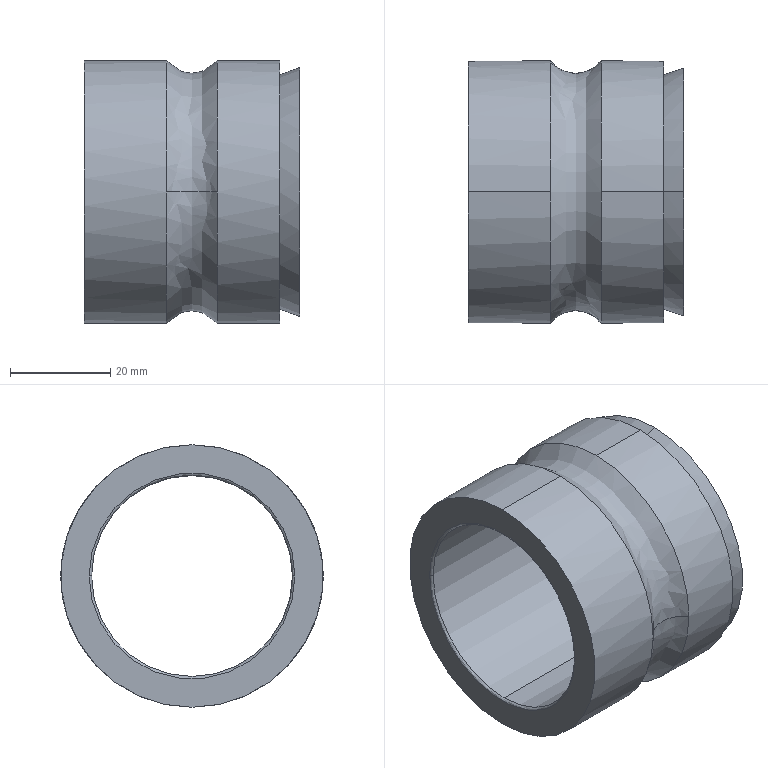Part | SolidWorks | features BaseBody 1 | 1 solid | 17 faces | box 42.9 x 52.3 x 52.3 mm | volume 34134 mm3 | spline 10 | cylinder 4 | plane 3 | commonest cylinder face diameters 52.3 x4
STEP:
#1=CARTESIAN_POINT('',(5.05,48.85,49.2));
#2=VERTEX_POINT('',#1);
#3=CARTESIAN_POINT('',(5.05,75.,23.05));
#4=VERTEX_POINT('',#3);
#5=CARTESIAN_POINT('',(5.05,75.,49.2));
#6=DIRECTION('',(1.,0.,0.));
#7=DIRECTION('',(0.,0.,1.));
#8=AXIS2_PLACEMENT_3D('',#5,#6,#7);
#9=CIRCLE('',#8,26.15);
#10=EDGE_CURVE('',#2,#4,#9,.T.);
#11=ORIENTED_EDGE('',*,*,#10,.F.);
#12=CARTESIAN_POINT('',(-5.05,48.85,49.2));
#13=VERTEX_POINT('',#12);
#14=CARTESIAN_POINT('',(0.,45.,49.2));
#15=DIRECTION('',(0.,0.,1.));
#16=DIRECTION('',(0.,-1.,0.));
#17=AXIS2_PLACEMENT_3D('',#14,#15,#16);
#18=CIRCLE('',#17,6.35);
#19=EDGE_CURVE('',#2,#13,#18,.T.);
#20=ORIENTED_EDGE('',*,*,#19,.T.);
#21=CARTESIAN_POINT('',(-5.05,75.,23.05));
#22=VERTEX_POINT('',#21);
#23=CARTESIAN_POINT('',(-5.05,75.,49.2));
#24=DIRECTION('',(1.,0.,0.));
#25=DIRECTION('',(0.,0.,1.));
#26=AXIS2_PLACEMENT_3D('',#23,#24,#25);
#27=CIRCLE('',#26,26.15);
#28=EDGE_CURVE('',#13,#22,#27,.T.);
#29=ORIENTED_EDGE('',*,*,#28,.T.);
#30=CARTESIAN_POINT('',(-5.05,101.15,49.2));
#31=VERTEX_POINT('',#30);
#32=CARTESIAN_POINT('',(-5.05,75.,49.2));
#33=DIRECTION('',(1.,0.,0.));
#34=DIRECTION('',(0.,0.,1.));
#35=AXIS2_PLACEMENT_3D('',#32,#33,#34);
#36=CIRCLE('',#35,26.15);
#37=EDGE_CURVE('',#22,#31,#36,.T.);
#38=ORIENTED_EDGE('',*,*,#37,.T.);
#39=CARTESIAN_POINT('',(5.05,101.15,49.2));
#40=VERTEX_POINT('',#39);
#41=CARTESIAN_POINT('',(0.,105.,49.2));
#42=DIRECTION('',(0.,0.,-1.));
#43=DIRECTION('',(0.,1.,0.));
#44=AXIS2_PLACEMENT_3D('',#41,#42,#43);
#45=CIRCLE('',#44,6.35);
#46=EDGE_CURVE('',#40,#31,#45,.T.);
#47=ORIENTED_EDGE('',*,*,#46,.F.);
#48=CARTESIAN_POINT('',(5.05,75.,49.2));
#49=DIRECTION('',(1.,0.,0.));
#50=DIRECTION('',(0.,0.,1.));
#51=AXIS2_PLACEMENT_3D('',#48,#49,#50);
#52=CIRCLE('',#51,26.15);
#53=EDGE_CURVE('',#4,#40,#52,.T.);
#54=ORIENTED_EDGE('',*,*,#53,.F.);
#55=EDGE_LOOP('',(#11,#20,#29,#38,#47,#54));
#56=FACE_OUTER_BOUND('',#55,.T.);
#57=CARTESIAN_POINT('',(5.05,48.85,49.2));
#58=CARTESIAN_POINT('',(5.05,48.85,-3.1));
#59=CARTESIAN_POINT('',(5.05,101.15,-3.1));
#60=CARTESIAN_POINT('',(5.05,101.15,49.2));
#61=CARTESIAN_POINT('',(2.282,52.48,49.2));
#62=CARTESIAN_POINT('',(2.282,52.48,4.16));
#63=CARTESIAN_POINT('',(2.282,97.52,4.16));
#64=CARTESIAN_POINT('',(2.282,97.52,49.2));
#65=CARTESIAN_POINT('',(-2.282,52.48,49.2));
#66=CARTESIAN_POINT('',(-2.282,52.48,4.16));
#67=CARTESIAN_POINT('',(-2.282,97.52,4.16));
#68=CARTESIAN_POINT('',(-2.282,97.52,49.2));
#69=CARTESIAN_POINT('',(-5.05,48.85,49.2));
#70=CARTESIAN_POINT('',(-5.05,48.85,-3.1));
#71=CARTESIAN_POINT('',(-5.05,101.15,-3.1));
#72=CARTESIAN_POINT('',(-5.05,101.15,49.2));
#73=(BOUNDED_SURFACE()B_SPLINE_SURFACE(3,3,((#57,#58,#59,#60),(#61,#62,#63,#64),(#65,#66,#67,#68),(#69,#70,#71,#72)),.UNSPECIFIED.,.F.,.F.,.F.)B_SPLINE_SURFACE_WITH_KNOTS((4,4),(4,4),(0.,1.),(0.,1.),.UNSPECIFIED.)GEOMETRIC_REPRESENTATION_ITEM()RATIONAL_B_SPLINE_SURFACE(((1.,0.3333,0.3333,1.),(0.7375,0.2458,0.2458,0.7375),(0.7375,0.2458,0.2458,0.7375),(1.,0.3333,0.3333,1.)))REPRESENTATION_ITEM('')SURFACE());
#74=ADVANCED_FACE('',(#56),#73,.T.);
#75=CARTESIAN_POINT('',(21.5,75.,24.419));
#76=VERTEX_POINT('',#75);
#77=CARTESIAN_POINT('',(21.5,75.,73.981));
#78=VERTEX_POINT('',#77);
#79=CARTESIAN_POINT('',(21.5,75.,49.2));
#80=DIRECTION('',(1.,0.,0.));
#81=DIRECTION('',(0.,0.,1.));
#82=AXIS2_PLACEMENT_3D('',#79,#80,#81);
#83=CIRCLE('',#82,24.781);
#84=EDGE_CURVE('',#76,#78,#83,.T.);
#85=ORIENTED_EDGE('',*,*,#84,.F.);
#86=CARTESIAN_POINT('',(17.5,75.,25.875));
#87=VERTEX_POINT('',#86);
#88=CARTESIAN_POINT('',(19.5,75.,25.147));
#89=DIRECTION('',(-0.9397,0.,0.342));
#90=VECTOR('',#89,1000.);
#91=LINE('',#88,#90);
#92=EDGE_CURVE('',#76,#87,#91,.T.);
#93=ORIENTED_EDGE('',*,*,#92,.T.);
#94=CARTESIAN_POINT('',(17.5,75.,72.525));
#95=VERTEX_POINT('',#94);
#96=CARTESIAN_POINT('',(17.5,75.,49.2));
#97=DIRECTION('',(1.,0.,0.));
#98=DIRECTION('',(0.,0.,1.));
#99=AXIS2_PLACEMENT_3D('',#96,#97,#98);
#100=CIRCLE('',#99,23.325);
#101=EDGE_CURVE('',#87,#95,#100,.T.);
#102=ORIENTED_EDGE('',*,*,#101,.T.);
#103=CARTESIAN_POINT('',(19.5,75.,73.253));
#104=DIRECTION('',(-0.9397,0.,-0.342));
#105=VECTOR('',#104,1000.);
#106=LINE('',#103,#105);
#107=EDGE_CURVE('',#78,#95,#106,.T.);
#108=ORIENTED_EDGE('',*,*,#107,.F.);
#109=EDGE_LOOP('',(#85,#93,#102,#108));
#110=FACE_OUTER_BOUND('',#109,.T.);
#111=CARTESIAN_POINT('',(21.5,75.,24.419));
#112=CARTESIAN_POINT('',(21.5,124.562,24.419));
#113=CARTESIAN_POINT('',(21.5,124.562,73.981));
#114=CARTESIAN_POINT('',(21.5,75.,73.981));
#115=CARTESIAN_POINT('',(17.5,75.,25.875));
#116=CARTESIAN_POINT('',(17.5,121.65,25.875));
#117=CARTESIAN_POINT('',(17.5,121.65,72.525));
#118=CARTESIAN_POINT('',(17.5,75.,72.525));
#119=(BOUNDED_SURFACE()B_SPLINE_SURFACE(1,3,((#111,#112,#113,#114),(#115,#116,#117,#118)),.UNSPECIFIED.,.F.,.F.,.F.)B_SPLINE_SURFACE_WITH_KNOTS((2,2),(4,4),(0.,1.),(0.,1.),.UNSPECIFIED.)GEOMETRIC_REPRESENTATION_ITEM()RATIONAL_B_SPLINE_SURFACE(((1.,0.3333,0.3333,1.),(1.,0.3333,0.3333,1.)))REPRESENTATION_ITEM('')SURFACE());
#120=ADVANCED_FACE('',(#110),#119,.T.);
#121=CARTESIAN_POINT('',(21.,55.,49.2));
#122=VERTEX_POINT('',#121);
#123=CARTESIAN_POINT('',(21.,75.,29.2));
#124=VERTEX_POINT('',#123);
#125=CARTESIAN_POINT('',(21.,75.,49.2));
#126=DIRECTION('',(1.,0.,0.));
#127=DIRECTION('',(0.,0.,1.));
#128=AXIS2_PLACEMENT_3D('',#125,#126,#127);
#129=CIRCLE('',#128,20.);
#130=EDGE_CURVE('',#122,#124,#129,.T.);
#131=ORIENTED_EDGE('',*,*,#130,.F.);
#132=CARTESIAN_POINT('',(21.5,54.5,49.2));
#133=VERTEX_POINT('',#132);
#134=CARTESIAN_POINT('',(21.,54.5,49.2));
#135=DIRECTION('',(0.,0.,-1.));
#136=DIRECTION('',(0.,-1.,0.));
#137=AXIS2_PLACEMENT_3D('',#134,#135,#136);
#138=CIRCLE('',#137,0.5);
#139=EDGE_CURVE('',#122,#133,#138,.T.);
#140=ORIENTED_EDGE('',*,*,#139,.T.);
#141=CARTESIAN_POINT('',(21.5,95.5,49.2));
#142=VERTEX_POINT('',#141);
#143=CARTESIAN_POINT('',(21.5,75.,49.2));
#144=DIRECTION('',(1.,0.,0.));
#145=DIRECTION('',(0.,0.,1.));
#146=AXIS2_PLACEMENT_3D('',#143,#144,#145);
#147=CIRCLE('',#146,20.5);
#148=EDGE_CURVE('',#133,#142,#147,.T.);
#149=ORIENTED_EDGE('',*,*,#148,.T.);
#150=CARTESIAN_POINT('',(21.,95.,49.2));
#151=VERTEX_POINT('',#150);
#152=CARTESIAN_POINT('',(21.,95.5,49.2));
#153=DIRECTION('',(0.,0.,1.));
#154=DIRECTION('',(0.,1.,0.));
#155=AXIS2_PLACEMENT_3D('',#152,#153,#154);
#156=CIRCLE('',#155,0.5);
#157=EDGE_CURVE('',#151,#142,#156,.T.);
#158=ORIENTED_EDGE('',*,*,#157,.F.);
#159=CARTESIAN_POINT('',(21.,75.,49.2));
#160=DIRECTION('',(1.,0.,0.));
#161=DIRECTION('',(0.,0.,1.));
#162=AXIS2_PLACEMENT_3D('',#159,#160,#161);
#163=CIRCLE('',#162,20.);
#164=EDGE_CURVE('',#124,#151,#163,.T.);
#165=ORIENTED_EDGE('',*,*,#164,.F.);
#166=EDGE_LOOP('',(#131,#140,#149,#158,#165));
#167=FACE_OUTER_BOUND('',#166,.T.);
#168=CARTESIAN_POINT('',(21.,55.,49.2));
#169=CARTESIAN_POINT('',(21.,55.,9.2));
#170=CARTESIAN_POINT('',(21.,95.,9.2));
#171=CARTESIAN_POINT('',(21.,95.,49.2));
#172=CARTESIAN_POINT('',(21.293,55.,49.2));
#173=CARTESIAN_POINT('',(21.293,55.,9.2));
#174=CARTESIAN_POINT('',(21.293,95.,9.2));
#175=CARTESIAN_POINT('',(21.293,95.,49.2));
#176=CARTESIAN_POINT('',(21.5,54.793,49.2));
#177=CARTESIAN_POINT('',(21.5,54.793,8.786));
#178=CARTESIAN_POINT('',(21.5,95.207,8.786));
#179=CARTESIAN_POINT('',(21.5,95.207,49.2));
#180=CARTESIAN_POINT('',(21.5,54.5,49.2));
#181=CARTESIAN_POINT('',(21.5,54.5,8.2));
#182=CARTESIAN_POINT('',(21.5,95.5,8.2));
#183=CARTESIAN_POINT('',(21.5,95.5,49.2));
#184=(BOUNDED_SURFACE()B_SPLINE_SURFACE(3,3,((#168,#169,#170,#171),(#172,#173,#174,#175),(#176,#177,#178,#179),(#180,#181,#182,#183)),.UNSPECIFIED.,.F.,.F.,.F.)B_SPLINE_SURFACE_WITH_KNOTS((4,4),(4,4),(0.,1.),(0.,1.),.UNSPECIFIED.)GEOMETRIC_REPRESENTATION_ITEM()RATIONAL_B_SPLINE_SURFACE(((1.,0.3333,0.3333,1.),(0.8047,0.2682,0.2682,0.8047),(0.8047,0.2682,0.2682,0.8047),(1.,0.3333,0.3333,1.)))REPRESENTATION_ITEM('')SURFACE());
#185=ADVANCED_FACE('',(#167),#184,.T.);
#186=CARTESIAN_POINT('',(-21.4,54.5,49.2));
#187=VERTEX_POINT('',#186);
#188=CARTESIAN_POINT('',(-21.4,95.5,49.2));
#189=VERTEX_POINT('',#188);
#190=CARTESIAN_POINT('',(-21.4,75.,49.2));
#191=DIRECTION('',(1.,0.,0.));
#192=DIRECTION('',(0.,0.,1.));
#193=AXIS2_PLACEMENT_3D('',#190,#191,#192);
#194=CIRCLE('',#193,20.5);
#195=EDGE_CURVE('',#187,#189,#194,.T.);
#196=ORIENTED_EDGE('',*,*,#195,.F.);
#197=CARTESIAN_POINT('',(-20.9,55.,49.2));
#198=VERTEX_POINT('',#197);
#199=CARTESIAN_POINT('',(-20.9,54.5,49.2));
#200=DIRECTION('',(0.,0.,-1.));
#201=DIRECTION('',(0.,-1.,0.));
#202=AXIS2_PLACEMENT_3D('',#199,#200,#201);
#203=CIRCLE('',#202,0.5);
#204=EDGE_CURVE('',#187,#198,#203,.T.);
#205=ORIENTED_EDGE('',*,*,#204,.T.);
#206=CARTESIAN_POINT('',(-20.9,75.,29.2));
#207=VERTEX_POINT('',#206);
#208=CARTESIAN_POINT('',(-20.9,75.,49.2));
#209=DIRECTION('',(1.,0.,0.));
#210=DIRECTION('',(0.,0.,1.));
#211=AXIS2_PLACEMENT_3D('',#208,#209,#210);
#212=CIRCLE('',#211,20.);
#213=EDGE_CURVE('',#198,#207,#212,.T.);
#214=ORIENTED_EDGE('',*,*,#213,.T.);
#215=CARTESIAN_POINT('',(-20.9,95.,49.2));
#216=VERTEX_POINT('',#215);
#217=CARTESIAN_POINT('',(-20.9,75.,49.2));
#218=DIRECTION('',(1.,0.,0.));
#219=DIRECTION('',(0.,0.,1.));
#220=AXIS2_PLACEMENT_3D('',#217,#218,#219);
#221=CIRCLE('',#220,20.);
#222=EDGE_CURVE('',#207,#216,#221,.T.);
#223=ORIENTED_EDGE('',*,*,#222,.T.);
#224=CARTESIAN_POINT('',(-20.9,95.5,49.2));
#225=DIRECTION('',(0.,0.,1.));
#226=DIRECTION('',(0.,1.,0.));
#227=AXIS2_PLACEMENT_3D('',#224,#225,#226);
#228=CIRCLE('',#227,0.5);
#229=EDGE_CURVE('',#189,#216,#228,.T.);
#230=ORIENTED_EDGE('',*,*,#229,.F.);
#231=EDGE_LOOP('',(#196,#205,#214,#223,#230));
#232=FACE_OUTER_BOUND('',#231,.T.);
#233=CARTESIAN_POINT('',(-21.4,54.5,49.2));
#234=CARTESIAN_POINT('',(-21.4,54.5,8.2));
#235=CARTESIAN_POINT('',(-21.4,95.5,8.2));
#236=CARTESIAN_POINT('',(-21.4,95.5,49.2));
#237=CARTESIAN_POINT('',(-21.4,54.793,49.2));
#238=CARTESIAN_POINT('',(-21.4,54.793,8.786));
#239=CARTESIAN_POINT('',(-21.4,95.207,8.786));
#240=CARTESIAN_POINT('',(-21.4,95.207,49.2));
#241=CARTESIAN_POINT('',(-21.193,55.,49.2));
#242=CARTESIAN_POINT('',(-21.193,55.,9.2));
#243=CARTESIAN_POINT('',(-21.193,95.,9.2));
#244=CARTESIAN_POINT('',(-21.193,95.,49.2));
#245=CARTESIAN_POINT('',(-20.9,55.,49.2));
#246=CARTESIAN_POINT('',(-20.9,55.,9.2));
#247=CARTESIAN_POINT('',(-20.9,95.,9.2));
#248=CARTESIAN_POINT('',(-20.9,95.,49.2));
#249=(BOUNDED_SURFACE()B_SPLINE_SURFACE(3,3,((#233,#234,#235,#236),(#237,#238,#239,#240),(#241,#242,#243,#244),(#245,#246,#247,#248)),.UNSPECIFIED.,.F.,.F.,.T.)B_SPLINE_SURFACE_WITH_KNOTS((4,4),(4,4),(0.,1.),(0.,1.),.UNSPECIFIED.)GEOMETRIC_REPRESENTATION_ITEM()RATIONAL_B_SPLINE_SURFACE(((1.,0.3333,0.3333,1.),(0.8047,0.2682,0.2682,0.8047),(0.8047,0.2682,0.2682,0.8047),(1.,0.3333,0.3333,1.)))REPRESENTATION_ITEM('')SURFACE());
#250=ADVANCED_FACE('',(#232),#249,.T.);
#251=CARTESIAN_POINT('',(-21.4,75.,23.05));
#252=VERTEX_POINT('',#251);
#253=CARTESIAN_POINT('',(-21.4,75.,75.35));
#254=VERTEX_POINT('',#253);
#255=CARTESIAN_POINT('',(-21.4,75.,49.2));
#256=DIRECTION('',(1.,0.,0.));
#257=DIRECTION('',(0.,0.,1.));
#258=AXIS2_PLACEMENT_3D('',#255,#256,#257);
#259=CIRCLE('',#258,26.15);
#260=EDGE_CURVE('',#252,#254,#259,.T.);
#261=ORIENTED_EDGE('',*,*,#260,.T.);
#262=CARTESIAN_POINT('',(-5.05,75.,75.35));
#263=VERTEX_POINT('',#262);
#264=CARTESIAN_POINT('',(-13.225,75.,75.35));
#265=DIRECTION('',(1.,0.,0.));
#266=VECTOR('',#265,1000.);
#267=LINE('',#264,#266);
#268=EDGE_CURVE('',#254,#263,#267,.T.);
#269=ORIENTED_EDGE('',*,*,#268,.T.);
#270=CARTESIAN_POINT('',(-5.05,75.,49.2));
#271=DIRECTION('',(1.,0.,0.));
#272=DIRECTION('',(0.,0.,1.));
#273=AXIS2_PLACEMENT_3D('',#270,#271,#272);
#274=CIRCLE('',#273,26.15);
#275=EDGE_CURVE('',#31,#263,#274,.T.);
#276=ORIENTED_EDGE('',*,*,#275,.F.);
#277=ORIENTED_EDGE('',*,*,#37,.F.);
#278=CARTESIAN_POINT('',(-13.225,75.,23.05));
#279=DIRECTION('',(1.,0.,0.));
#280=VECTOR('',#279,1000.);
#281=LINE('',#278,#280);
#282=EDGE_CURVE('',#252,#22,#281,.T.);
#283=ORIENTED_EDGE('',*,*,#282,.F.);
#284=EDGE_LOOP('',(#261,#269,#276,#277,#283));
#285=FACE_OUTER_BOUND('',#284,.T.);
#286=CARTESIAN_POINT('',(-13.225,75.,49.2));
#287=DIRECTION('',(1.,0.,0.));
#288=DIRECTION('',(0.,0.,-1.));
#289=AXIS2_PLACEMENT_3D('',#286,#287,#288);
#290=CYLINDRICAL_SURFACE('',#289,26.15);
#291=ADVANCED_FACE('',(#285),#290,.T.);
#292=ORIENTED_EDGE('',*,*,#53,.T.);
#293=CARTESIAN_POINT('',(5.05,75.,75.35));
#294=VERTEX_POINT('',#293);
#295=CARTESIAN_POINT('',(5.05,75.,49.2));
#296=DIRECTION('',(1.,0.,0.));
#297=DIRECTION('',(0.,0.,1.));
#298=AXIS2_PLACEMENT_3D('',#295,#296,#297);
#299=CIRCLE('',#298,26.15);
#300=EDGE_CURVE('',#40,#294,#299,.T.);
#301=ORIENTED_EDGE('',*,*,#300,.T.);
#302=CARTESIAN_POINT('',(17.5,75.,75.35));
#303=VERTEX_POINT('',#302);
#304=CARTESIAN_POINT('',(11.275,75.,75.35));
#305=DIRECTION('',(1.,0.,0.));
#306=VECTOR('',#305,1000.);
#307=LINE('',#304,#306);
#308=EDGE_CURVE('',#294,#303,#307,.T.);
#309=ORIENTED_EDGE('',*,*,#308,.T.);
#310=CARTESIAN_POINT('',(17.5,75.,23.05));
#311=VERTEX_POINT('',#310);
#312=CARTESIAN_POINT('',(17.5,75.,49.2));
#313=DIRECTION('',(1.,0.,0.));
#314=DIRECTION('',(0.,0.,1.));
#315=AXIS2_PLACEMENT_3D('',#312,#313,#314);
#316=CIRCLE('',#315,26.15);
#317=EDGE_CURVE('',#311,#303,#316,.T.);
#318=ORIENTED_EDGE('',*,*,#317,.F.);
#319=CARTESIAN_POINT('',(11.275,75.,23.05));
#320=DIRECTION('',(1.,0.,0.));
#321=VECTOR('',#320,1000.);
#322=LINE('',#319,#321);
#323=EDGE_CURVE('',#4,#311,#322,.T.);
#324=ORIENTED_EDGE('',*,*,#323,.F.);
#325=EDGE_LOOP('',(#292,#301,#309,#318,#324));
#326=FACE_OUTER_BOUND('',#325,.T.);
#327=CARTESIAN_POINT('',(11.275,75.,49.2));
#328=DIRECTION('',(1.,0.,0.));
#329=DIRECTION('',(0.,0.,-1.));
#330=AXIS2_PLACEMENT_3D('',#327,#328,#329);
#331=CYLINDRICAL_SURFACE('',#330,26.15);
#332=ADVANCED_FACE('',(#326),#331,.T.);
#333=ORIENTED_EDGE('',*,*,#222,.F.);
#334=CARTESIAN_POINT('',(0.05,75.,29.2));
#335=DIRECTION('',(1.,0.,0.));
#336=VECTOR('',#335,1000.);
#337=LINE('',#334,#336);
#338=EDGE_CURVE('',#207,#124,#337,.T.);
#339=ORIENTED_EDGE('',*,*,#338,.T.);
#340=ORIENTED_EDGE('',*,*,#164,.T.);
#341=CARTESIAN_POINT('',(21.,75.,69.2));
#342=VERTEX_POINT('',#341);
#343=CARTESIAN_POINT('',(21.,75.,49.2));
#344=DIRECTION('',(1.,0.,0.));
#345=DIRECTION('',(0.,0.,1.));
#346=AXIS2_PLACEMENT_3D('',#343,#344,#345);
#347=CIRCLE('',#346,20.);
#348=EDGE_CURVE('',#151,#342,#347,.T.);
#349=ORIENTED_EDGE('',*,*,#348,.T.);
#350=CARTESIAN_POINT('',(-20.9,75.,69.2));
#351=VERTEX_POINT('',#350);
#352=CARTESIAN_POINT('',(0.05,75.,69.2));
#353=DIRECTION('',(1.,0.,0.));
#354=VECTOR('',#353,1000.);
#355=LINE('',#352,#354);
#356=EDGE_CURVE('',#351,#342,#355,.T.);
#357=ORIENTED_EDGE('',*,*,#356,.F.);
#358=CARTESIAN_POINT('',(-20.9,75.,49.2));
#359=DIRECTION('',(1.,0.,0.));
#360=DIRECTION('',(0.,0.,1.));
#361=AXIS2_PLACEMENT_3D('',#358,#359,#360);
#362=CIRCLE('',#361,20.);
#363=EDGE_CURVE('',#216,#351,#362,.T.);
#364=ORIENTED_EDGE('',*,*,#363,.F.);
#365=EDGE_LOOP('',(#333,#339,#340,#349,#357,#364));
#366=FACE_OUTER_BOUND('',#365,.T.);
#367=CARTESIAN_POINT('',(-20.9,75.,69.2));
#368=CARTESIAN_POINT('',(21.,75.,69.2));
#369=CARTESIAN_POINT('',(-20.9,115.,69.2));
#370=CARTESIAN_POINT('',(21.,115.,69.2));
#371=CARTESIAN_POINT('',(-20.9,115.,29.2));
#372=CARTESIAN_POINT('',(21.,115.,29.2));
#373=CARTESIAN_POINT('',(-20.9,75.,29.2));
#374=CARTESIAN_POINT('',(21.,75.,29.2));
#375=(BOUNDED_SURFACE()B_SPLINE_SURFACE(3,1,((#367,#368),(#369,#370),(#371,#372),(#373,#374)),.UNSPECIFIED.,.F.,.F.,.F.)B_SPLINE_SURFACE_WITH_KNOTS((4,4),(2,2),(0.,1.),(0.,1.),.UNSPECIFIED.)GEOMETRIC_REPRESENTATION_ITEM()RATIONAL_B_SPLINE_SURFACE(((1.,1.),(0.3333,0.3333),(0.3333,0.3333),(1.,1.)))REPRESENTATION_ITEM('')SURFACE());
#376=ADVANCED_FACE('',(#366),#375,.T.);
#377=CARTESIAN_POINT('',(-21.4,75.,49.2));
#378=DIRECTION('',(1.,0.,0.));
#379=DIRECTION('',(0.,0.,1.));
#380=AXIS2_PLACEMENT_3D('',#377,#378,#379);
#381=CIRCLE('',#380,20.5);
#382=EDGE_CURVE('',#189,#187,#381,.T.);
#383=ORIENTED_EDGE('',*,*,#382,.T.);
#384=ORIENTED_EDGE('',*,*,#195,.T.);
#385=EDGE_LOOP('',(#383,#384));
#386=FACE_BOUND('',#385,.T.);
#387=ORIENTED_EDGE('',*,*,#260,.F.);
#388=CARTESIAN_POINT('',(-21.4,75.,49.2));
#389=DIRECTION('',(1.,0.,0.));
#390=DIRECTION('',(0.,0.,1.));
#391=AXIS2_PLACEMENT_3D('',#388,#389,#390);
#392=CIRCLE('',#391,26.15);
#393=EDGE_CURVE('',#254,#252,#392,.T.);
#394=ORIENTED_EDGE('',*,*,#393,.F.);
#395=EDGE_LOOP('',(#387,#394));
#396=FACE_OUTER_BOUND('',#395,.T.);
#397=CARTESIAN_POINT('',(-21.4,75.,72.525));
#398=DIRECTION('',(-1.,0.,0.));
#399=DIRECTION('',(0.,0.,1.));
#400=AXIS2_PLACEMENT_3D('',#397,#398,#399);
#401=PLANE('',#400);
#402=ADVANCED_FACE('',(#386,#396),#401,.T.);
#403=ORIENTED_EDGE('',*,*,#204,.F.);
#404=ORIENTED_EDGE('',*,*,#382,.F.);
#405=ORIENTED_EDGE('',*,*,#229,.T.);
#406=ORIENTED_EDGE('',*,*,#363,.T.);
#407=CARTESIAN_POINT('',(-20.9,75.,49.2));
#408=DIRECTION('',(1.,0.,0.));
#409=DIRECTION('',(0.,0.,1.));
#410=AXIS2_PLACEMENT_3D('',#407,#408,#409);
#411=CIRCLE('',#410,20.);
#412=EDGE_CURVE('',#351,#198,#411,.T.);
#413=ORIENTED_EDGE('',*,*,#412,.T.);
#414=EDGE_LOOP('',(#403,#404,#405,#406,#413));
#415=FACE_OUTER_BOUND('',#414,.T.);
#416=CARTESIAN_POINT('',(-21.4,95.5,49.2));
#417=CARTESIAN_POINT('',(-21.4,95.5,90.2));
#418=CARTESIAN_POINT('',(-21.4,54.5,90.2));
#419=CARTESIAN_POINT('',(-21.4,54.5,49.2));
#420=CARTESIAN_POINT('',(-21.4,95.207,49.2));
#421=CARTESIAN_POINT('',(-21.4,95.207,89.614));
#422=CARTESIAN_POINT('',(-21.4,54.793,89.614));
#423=CARTESIAN_POINT('',(-21.4,54.793,49.2));
#424=CARTESIAN_POINT('',(-21.193,95.,49.2));
#425=CARTESIAN_POINT('',(-21.193,95.,89.2));
#426=CARTESIAN_POINT('',(-21.193,55.,89.2));
#427=CARTESIAN_POINT('',(-21.193,55.,49.2));
#428=CARTESIAN_POINT('',(-20.9,95.,49.2));
#429=CARTESIAN_POINT('',(-20.9,95.,89.2));
#430=CARTESIAN_POINT('',(-20.9,55.,89.2));
#431=CARTESIAN_POINT('',(-20.9,55.,49.2));
#432=(BOUNDED_SURFACE()B_SPLINE_SURFACE(3,3,((#416,#417,#418,#419),(#420,#421,#422,#423),(#424,#425,#426,#427),(#428,#429,#430,#431)),.UNSPECIFIED.,.F.,.F.,.F.)B_SPLINE_SURFACE_WITH_KNOTS((4,4),(4,4),(0.,1.),(0.,1.),.UNSPECIFIED.)GEOMETRIC_REPRESENTATION_ITEM()RATIONAL_B_SPLINE_SURFACE(((1.,0.3333,0.3333,1.),(0.8047,0.2682,0.2682,0.8047),(0.8047,0.2682,0.2682,0.8047),(1.,0.3333,0.3333,1.)))REPRESENTATION_ITEM('')SURFACE());
#433=ADVANCED_FACE('',(#415),#432,.T.);
#434=ORIENTED_EDGE('',*,*,#338,.F.);
#435=ORIENTED_EDGE('',*,*,#213,.F.);
#436=ORIENTED_EDGE('',*,*,#412,.F.);
#437=ORIENTED_EDGE('',*,*,#356,.T.);
#438=CARTESIAN_POINT('',(21.,75.,49.2));
#439=DIRECTION('',(1.,0.,0.));
#440=DIRECTION('',(0.,0.,1.));
#441=AXIS2_PLACEMENT_3D('',#438,#439,#440);
#442=CIRCLE('',#441,20.);
#443=EDGE_CURVE('',#342,#122,#442,.T.);
#444=ORIENTED_EDGE('',*,*,#443,.T.);
#445=ORIENTED_EDGE('',*,*,#130,.T.);
#446=EDGE_LOOP('',(#434,#435,#436,#437,#444,#445));
#447=FACE_OUTER_BOUND('',#446,.T.);
#448=CARTESIAN_POINT('',(-20.9,75.,29.2));
#449=CARTESIAN_POINT('',(21.,75.,29.2));
#450=CARTESIAN_POINT('',(-20.9,35.,29.2));
#451=CARTESIAN_POINT('',(21.,35.,29.2));
#452=CARTESIAN_POINT('',(-20.9,35.,69.2));
#453=CARTESIAN_POINT('',(21.,35.,69.2));
#454=CARTESIAN_POINT('',(-20.9,75.,69.2));
#455=CARTESIAN_POINT('',(21.,75.,69.2));
#456=(BOUNDED_SURFACE()B_SPLINE_SURFACE(3,1,((#448,#449),(#450,#451),(#452,#453),(#454,#455)),.UNSPECIFIED.,.F.,.F.,.F.)B_SPLINE_SURFACE_WITH_KNOTS((4,4),(2,2),(0.,1.),(0.,1.),.UNSPECIFIED.)GEOMETRIC_REPRESENTATION_ITEM()RATIONAL_B_SPLINE_SURFACE(((1.,1.),(0.3333,0.3333),(0.3333,0.3333),(1.,1.)))REPRESENTATION_ITEM('')SURFACE());
#457=ADVANCED_FACE('',(#447),#456,.T.);
#458=ORIENTED_EDGE('',*,*,#139,.F.);
#459=ORIENTED_EDGE('',*,*,#443,.F.);
#460=ORIENTED_EDGE('',*,*,#348,.F.);
#461=ORIENTED_EDGE('',*,*,#157,.T.);
#462=CARTESIAN_POINT('',(21.5,75.,49.2));
#463=DIRECTION('',(1.,0.,0.));
#464=DIRECTION('',(0.,0.,1.));
#465=AXIS2_PLACEMENT_3D('',#462,#463,#464);
#466=CIRCLE('',#465,20.5);
#467=EDGE_CURVE('',#142,#133,#466,.T.);
#468=ORIENTED_EDGE('',*,*,#467,.T.);
#469=EDGE_LOOP('',(#458,#459,#460,#461,#468));
#470=FACE_OUTER_BOUND('',#469,.T.);
#471=CARTESIAN_POINT('',(21.,95.,49.2));
#472=CARTESIAN_POINT('',(21.,95.,89.2));
#473=CARTESIAN_POINT('',(21.,55.,89.2));
#474=CARTESIAN_POINT('',(21.,55.,49.2));
#475=CARTESIAN_POINT('',(21.293,95.,49.2));
#476=CARTESIAN_POINT('',(21.293,95.,89.2));
#477=CARTESIAN_POINT('',(21.293,55.,89.2));
#478=CARTESIAN_POINT('',(21.293,55.,49.2));
#479=CARTESIAN_POINT('',(21.5,95.207,49.2));
#480=CARTESIAN_POINT('',(21.5,95.207,89.614));
#481=CARTESIAN_POINT('',(21.5,54.793,89.614));
#482=CARTESIAN_POINT('',(21.5,54.793,49.2));
#483=CARTESIAN_POINT('',(21.5,95.5,49.2));
#484=CARTESIAN_POINT('',(21.5,95.5,90.2));
#485=CARTESIAN_POINT('',(21.5,54.5,90.2));
#486=CARTESIAN_POINT('',(21.5,54.5,49.2));
#487=(BOUNDED_SURFACE()B_SPLINE_SURFACE(3,3,((#471,#472,#473,#474),(#475,#476,#477,#478),(#479,#480,#481,#482),(#483,#484,#485,#486)),.UNSPECIFIED.,.F.,.F.,.F.)B_SPLINE_SURFACE_WITH_KNOTS((4,4),(4,4),(0.,1.),(0.,1.),.UNSPECIFIED.)GEOMETRIC_REPRESENTATION_ITEM()RATIONAL_B_SPLINE_SURFACE(((1.,0.3333,0.3333,1.),(0.8047,0.2682,0.2682,0.8047),(0.8047,0.2682,0.2682,0.8047),(1.,0.3333,0.3333,1.)))REPRESENTATION_ITEM('')SURFACE());
#488=ADVANCED_FACE('',(#470),#487,.T.);
#489=CARTESIAN_POINT('',(21.5,75.,49.2));
#490=DIRECTION('',(1.,0.,0.));
#491=DIRECTION('',(0.,0.,1.));
#492=AXIS2_PLACEMENT_3D('',#489,#490,#491);
#493=CIRCLE('',#492,24.781);
#494=EDGE_CURVE('',#78,#76,#493,.T.);
#495=ORIENTED_EDGE('',*,*,#494,.T.);
#496=ORIENTED_EDGE('',*,*,#84,.T.);
#497=EDGE_LOOP('',(#495,#496));
#498=FACE_OUTER_BOUND('',#497,.T.);
#499=ORIENTED_EDGE('',*,*,#467,.F.);
#500=ORIENTED_EDGE('',*,*,#148,.F.);
#501=EDGE_LOOP('',(#499,#500));
#502=FACE_BOUND('',#501,.T.);
#503=CARTESIAN_POINT('',(21.5,75.,71.84));
#504=DIRECTION('',(1.,0.,0.));
#505=DIRECTION('',(0.,0.,-1.));
#506=AXIS2_PLACEMENT_3D('',#503,#504,#505);
#507=PLANE('',#506);
#508=ADVANCED_FACE('',(#498,#502),#507,.T.);
#509=ORIENTED_EDGE('',*,*,#92,.F.);
#510=ORIENTED_EDGE('',*,*,#494,.F.);
#511=ORIENTED_EDGE('',*,*,#107,.T.);
#512=CARTESIAN_POINT('',(17.5,75.,49.2));
#513=DIRECTION('',(1.,0.,0.));
#514=DIRECTION('',(0.,0.,1.));
#515=AXIS2_PLACEMENT_3D('',#512,#513,#514);
#516=CIRCLE('',#515,23.325);
#517=EDGE_CURVE('',#95,#87,#516,.T.);
#518=ORIENTED_EDGE('',*,*,#517,.T.);
#519=EDGE_LOOP('',(#509,#510,#511,#518));
#520=FACE_OUTER_BOUND('',#519,.T.);
#521=CARTESIAN_POINT('',(21.5,75.,73.981));
#522=CARTESIAN_POINT('',(21.5,25.438,73.981));
#523=CARTESIAN_POINT('',(21.5,25.438,24.419));
#524=CARTESIAN_POINT('',(21.5,75.,24.419));
#525=CARTESIAN_POINT('',(17.5,75.,72.525));
#526=CARTESIAN_POINT('',(17.5,28.35,72.525));
#527=CARTESIAN_POINT('',(17.5,28.35,25.875));
#528=CARTESIAN_POINT('',(17.5,75.,25.875));
#529=(BOUNDED_SURFACE()B_SPLINE_SURFACE(1,3,((#521,#522,#523,#524),(#525,#526,#527,#528)),.UNSPECIFIED.,.F.,.F.,.F.)B_SPLINE_SURFACE_WITH_KNOTS((2,2),(4,4),(0.,1.),(0.,1.),.UNSPECIFIED.)GEOMETRIC_REPRESENTATION_ITEM()RATIONAL_B_SPLINE_SURFACE(((1.,0.3333,0.3333,1.),(1.,0.3333,0.3333,1.)))REPRESENTATION_ITEM('')SURFACE());
#530=ADVANCED_FACE('',(#520),#529,.T.);
#531=ORIENTED_EDGE('',*,*,#317,.T.);
#532=CARTESIAN_POINT('',(17.5,75.,49.2));
#533=DIRECTION('',(1.,0.,0.));
#534=DIRECTION('',(0.,0.,1.));
#535=AXIS2_PLACEMENT_3D('',#532,#533,#534);
#536=CIRCLE('',#535,26.15);
#537=EDGE_CURVE('',#303,#311,#536,.T.);
#538=ORIENTED_EDGE('',*,*,#537,.T.);
#539=EDGE_LOOP('',(#531,#538));
#540=FACE_OUTER_BOUND('',#539,.T.);
#541=ORIENTED_EDGE('',*,*,#517,.F.);
#542=ORIENTED_EDGE('',*,*,#101,.F.);
#543=EDGE_LOOP('',(#541,#542));
#544=FACE_BOUND('',#543,.T.);
#545=CARTESIAN_POINT('',(17.5,75.,73.938));
#546=DIRECTION('',(1.,0.,0.));
#547=DIRECTION('',(0.,0.,-1.));
#548=AXIS2_PLACEMENT_3D('',#545,#546,#547);
#549=PLANE('',#548);
#550=ADVANCED_FACE('',(#540,#544),#549,.T.);
#551=ORIENTED_EDGE('',*,*,#308,.F.);
#552=CARTESIAN_POINT('',(5.05,75.,49.2));
#553=DIRECTION('',(1.,0.,0.));
#554=DIRECTION('',(0.,0.,1.));
#555=AXIS2_PLACEMENT_3D('',#552,#553,#554);
#556=CIRCLE('',#555,26.15);
#557=EDGE_CURVE('',#294,#2,#556,.T.);
#558=ORIENTED_EDGE('',*,*,#557,.T.);
#559=ORIENTED_EDGE('',*,*,#10,.T.);
#560=ORIENTED_EDGE('',*,*,#323,.T.);
#561=ORIENTED_EDGE('',*,*,#537,.F.);
#562=EDGE_LOOP('',(#551,#558,#559,#560,#561));
#563=FACE_OUTER_BOUND('',#562,.T.);
#564=CARTESIAN_POINT('',(11.275,75.,49.2));
#565=DIRECTION('',(1.,0.,0.));
#566=DIRECTION('',(0.,0.,-1.));
#567=AXIS2_PLACEMENT_3D('',#564,#565,#566);
#568=CYLINDRICAL_SURFACE('',#567,26.15);
#569=ADVANCED_FACE('',(#563),#568,.T.);
#570=ORIENTED_EDGE('',*,*,#19,.F.);
#571=ORIENTED_EDGE('',*,*,#557,.F.);
#572=ORIENTED_EDGE('',*,*,#300,.F.);
#573=ORIENTED_EDGE('',*,*,#46,.T.);
#574=ORIENTED_EDGE('',*,*,#275,.T.);
#575=CARTESIAN_POINT('',(-5.05,75.,49.2));
#576=DIRECTION('',(1.,0.,0.));
#577=DIRECTION('',(0.,0.,1.));
#578=AXIS2_PLACEMENT_3D('',#575,#576,#577);
#579=CIRCLE('',#578,26.15);
#580=EDGE_CURVE('',#263,#13,#579,.T.);
#581=ORIENTED_EDGE('',*,*,#580,.T.);
#582=EDGE_LOOP('',(#570,#571,#572,#573,#574,#581));
#583=FACE_OUTER_BOUND('',#582,.T.);
#584=CARTESIAN_POINT('',(5.05,101.15,49.2));
#585=CARTESIAN_POINT('',(5.05,101.15,101.5));
#586=CARTESIAN_POINT('',(5.05,48.85,101.5));
#587=CARTESIAN_POINT('',(5.05,48.85,49.2));
#588=CARTESIAN_POINT('',(2.282,97.52,49.2));
#589=CARTESIAN_POINT('',(2.282,97.52,94.24));
#590=CARTESIAN_POINT('',(2.282,52.48,94.24));
#591=CARTESIAN_POINT('',(2.282,52.48,49.2));
#592=CARTESIAN_POINT('',(-2.282,97.52,49.2));
#593=CARTESIAN_POINT('',(-2.282,97.52,94.24));
#594=CARTESIAN_POINT('',(-2.282,52.48,94.24));
#595=CARTESIAN_POINT('',(-2.282,52.48,49.2));
#596=CARTESIAN_POINT('',(-5.05,101.15,49.2));
#597=CARTESIAN_POINT('',(-5.05,101.15,101.5));
#598=CARTESIAN_POINT('',(-5.05,48.85,101.5));
#599=CARTESIAN_POINT('',(-5.05,48.85,49.2));
#600=(BOUNDED_SURFACE()B_SPLINE_SURFACE(3,3,((#584,#585,#586,#587),(#588,#589,#590,#591),(#592,#593,#594,#595),(#596,#597,#598,#599)),.UNSPECIFIED.,.F.,.F.,.F.)B_SPLINE_SURFACE_WITH_KNOTS((4,4),(4,4),(0.,1.),(0.,1.),.UNSPECIFIED.)GEOMETRIC_REPRESENTATION_ITEM()RATIONAL_B_SPLINE_SURFACE(((1.,0.3333,0.3333,1.),(0.7375,0.2458,0.2458,0.7375),(0.7375,0.2458,0.2458,0.7375),(1.,0.3333,0.3333,1.)))REPRESENTATION_ITEM('')SURFACE());
#601=ADVANCED_FACE('',(#583),#600,.T.);
#602=ORIENTED_EDGE('',*,*,#268,.F.);
#603=ORIENTED_EDGE('',*,*,#393,.T.);
#604=ORIENTED_EDGE('',*,*,#282,.T.);
#605=ORIENTED_EDGE('',*,*,#28,.F.);
#606=ORIENTED_EDGE('',*,*,#580,.F.);
#607=EDGE_LOOP('',(#602,#603,#604,#605,#606));
#608=FACE_OUTER_BOUND('',#607,.T.);
#609=CARTESIAN_POINT('',(-13.225,75.,49.2));
#610=DIRECTION('',(1.,0.,0.));
#611=DIRECTION('',(0.,0.,-1.));
#612=AXIS2_PLACEMENT_3D('',#609,#610,#611);
#613=CYLINDRICAL_SURFACE('',#612,26.15);
#614=ADVANCED_FACE('',(#608),#613,.T.);
#615=CLOSED_SHELL('',(#74,#120,#185,#250,#291,#332,#376,#402,#433,#457,#488,#508,#530,#550,#569,#601,#614));
#616=MANIFOLD_SOLID_BREP('',#615);
#617=CARTESIAN_POINT('',(0.,0.,0.));
#618=DIRECTION('',(0.,0.,1.));
#619=DIRECTION('',(1.,0.,0.));
#620=AXIS2_PLACEMENT_3D('',#617,#618,#619);
#621=(LENGTH_UNIT()NAMED_UNIT(*)SI_UNIT(.MILLI.,.METRE.));
#622=UNCERTAINTY_MEASURE_WITH_UNIT(LENGTH_MEASURE(0.00001),#621,'','');
#623=(NAMED_UNIT(*)PLANE_ANGLE_UNIT()SI_UNIT($,.RADIAN.));
#624=(NAMED_UNIT(*)SI_UNIT($,.STERADIAN.)SOLID_ANGLE_UNIT());
#625=(GEOMETRIC_REPRESENTATION_CONTEXT(3)GLOBAL_UNCERTAINTY_ASSIGNED_CONTEXT((#622))GLOBAL_UNIT_ASSIGNED_CONTEXT((#621,#623,#624))REPRESENTATION_CONTEXT('',''));
#626=ADVANCED_BREP_SHAPE_REPRESENTATION('',(#616,#620),#625);